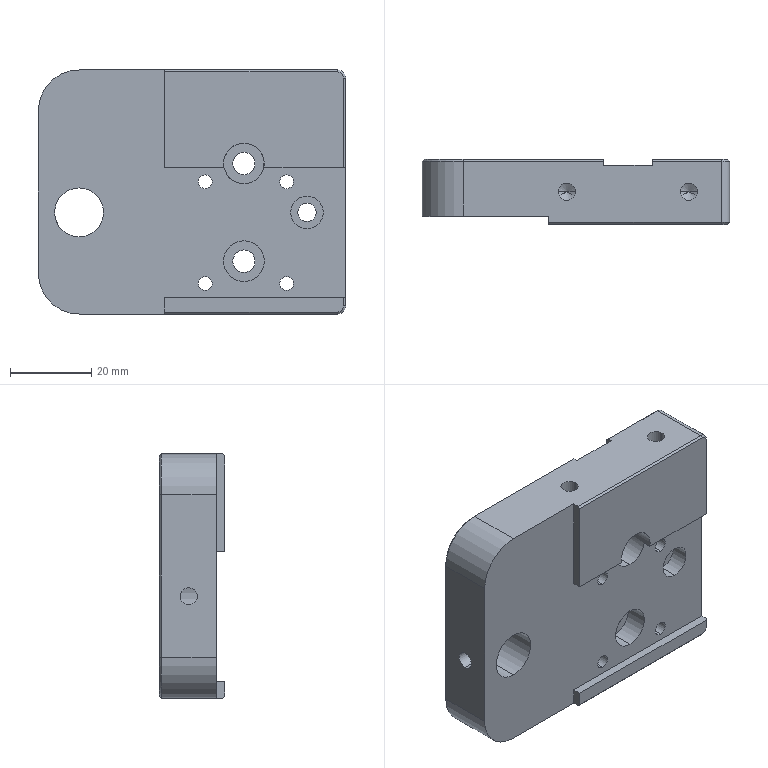Part | STEP file | ND25021-01-JDKM-52-TL | 1 solid | 84 faces | box 75.5 x 16 x 60 mm | volume 59527 mm3 | cylinder 40 | plane 34 | cone 10 | commonest cylinder face diameters 3.4 x8 6 x8 4.2 x6 5.5 x4 10 x4 4 x2